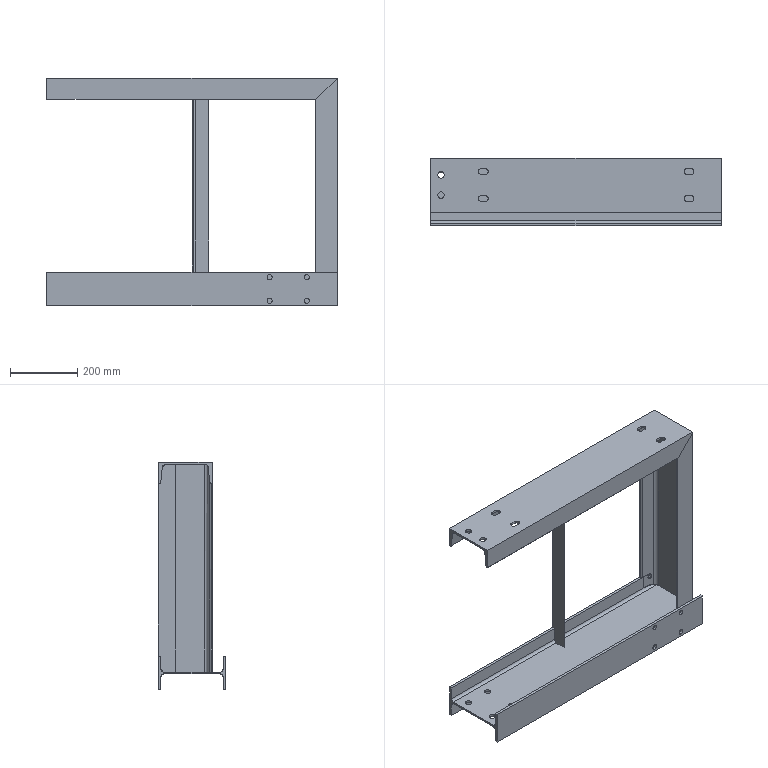Part | STEP file | Transfer kettle landing body_Default<As Machined> | 4 solids | 110 faces | box 860 x 200 x 675 mm | volume 5631286 mm3 | plane 59 | cylinder 51 | commonest cylinder face diameters 19 x24 15 x8 10 x4 13 x4 16 x4 20 x4